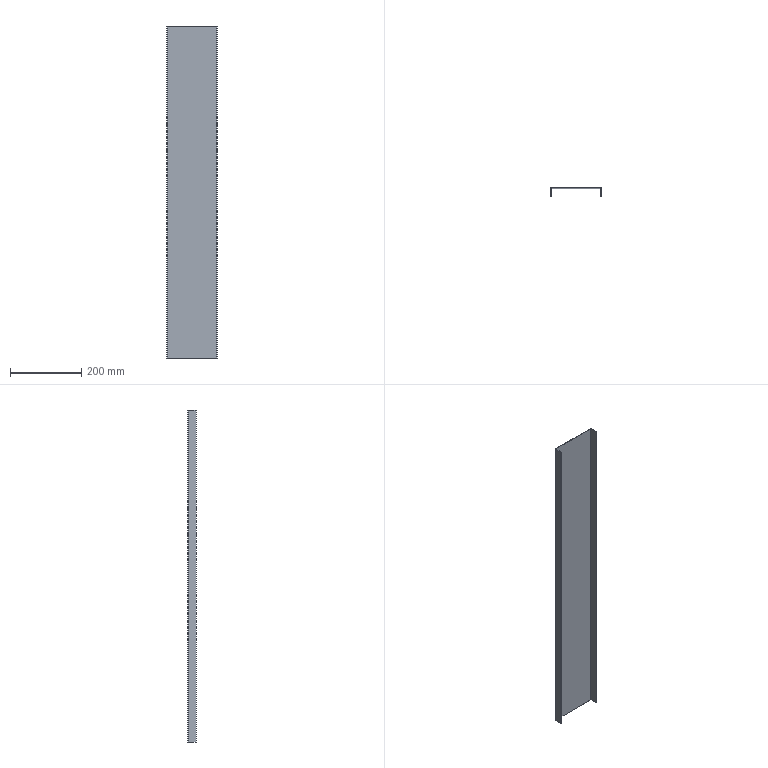Part | 1 solid | 22 faces | box 142 x 23 x 935 mm | volume 172917 mm3 | plane 18 | cylinder 4 | commonest cylinder face diameters 1.473 x2 3.473 x2
STEP:
#1=CARTESIAN_POINT('',(69.263,22.,935.));
#2=VERTEX_POINT('',#1);
#3=CARTESIAN_POINT('',(69.263,23.,935.));
#4=VERTEX_POINT('',#3);
#5=CARTESIAN_POINT('',(69.263,22.,935.));
#6=DIRECTION('',(0.,1.,0.));
#7=VECTOR('',#6,1000.);
#8=LINE('',#5,#7);
#9=EDGE_CURVE('',#2,#4,#8,.T.);
#10=ORIENTED_EDGE('',*,*,#9,.F.);
#11=CARTESIAN_POINT('',(70.,21.263,935.));
#12=VERTEX_POINT('',#11);
#13=CARTESIAN_POINT('',(69.263,21.263,935.));
#14=DIRECTION('',(0.,0.,1.));
#15=DIRECTION('',(-1.,0.,0.));
#16=AXIS2_PLACEMENT_3D('',#13,#14,#15);
#17=CIRCLE('',#16,0.7366);
#18=EDGE_CURVE('',#12,#2,#17,.T.);
#19=ORIENTED_EDGE('',*,*,#18,.F.);
#20=CARTESIAN_POINT('',(71.,21.263,935.));
#21=VERTEX_POINT('',#20);
#22=CARTESIAN_POINT('',(71.,21.263,935.));
#23=DIRECTION('',(-1.,0.,0.));
#24=VECTOR('',#23,1000.);
#25=LINE('',#22,#24);
#26=EDGE_CURVE('',#21,#12,#25,.T.);
#27=ORIENTED_EDGE('',*,*,#26,.F.);
#28=CARTESIAN_POINT('',(69.263,21.263,935.));
#29=DIRECTION('',(0.,0.,1.));
#30=DIRECTION('',(1.,0.,0.));
#31=AXIS2_PLACEMENT_3D('',#28,#29,#30);
#32=CIRCLE('',#31,1.737);
#33=EDGE_CURVE('',#21,#4,#32,.T.);
#34=ORIENTED_EDGE('',*,*,#33,.T.);
#35=EDGE_LOOP('',(#10,#19,#27,#34));
#36=FACE_OUTER_BOUND('',#35,.T.);
#37=CARTESIAN_POINT('',(69.263,22.,935.));
#38=DIRECTION('',(0.,0.,1.));
#39=DIRECTION('',(1.,0.,0.));
#40=AXIS2_PLACEMENT_3D('',#37,#38,#39);
#41=PLANE('',#40);
#42=ADVANCED_FACE('',(#36),#41,.T.);
#43=CARTESIAN_POINT('',(-69.263,22.,935.));
#44=VERTEX_POINT('',#43);
#45=CARTESIAN_POINT('',(-70.,22.,935.));
#46=DIRECTION('',(-1.,0.,0.));
#47=VECTOR('',#46,1000.);
#48=LINE('',#45,#47);
#49=EDGE_CURVE('',#2,#44,#48,.T.);
#50=ORIENTED_EDGE('',*,*,#49,.F.);
#51=ORIENTED_EDGE('',*,*,#9,.T.);
#52=CARTESIAN_POINT('',(-69.263,23.,935.));
#53=VERTEX_POINT('',#52);
#54=CARTESIAN_POINT('',(-70.,23.,935.));
#55=DIRECTION('',(-1.,0.,0.));
#56=VECTOR('',#55,1000.);
#57=LINE('',#54,#56);
#58=EDGE_CURVE('',#4,#53,#57,.T.);
#59=ORIENTED_EDGE('',*,*,#58,.T.);
#60=CARTESIAN_POINT('',(-69.263,23.,935.));
#61=DIRECTION('',(0.,-1.,0.));
#62=VECTOR('',#61,1000.);
#63=LINE('',#60,#62);
#64=EDGE_CURVE('',#53,#44,#63,.T.);
#65=ORIENTED_EDGE('',*,*,#64,.T.);
#66=EDGE_LOOP('',(#50,#51,#59,#65));
#67=FACE_OUTER_BOUND('',#66,.T.);
#68=CARTESIAN_POINT('',(71.,21.263,935.));
#69=DIRECTION('',(0.,0.,1.));
#70=DIRECTION('',(1.,0.,0.));
#71=AXIS2_PLACEMENT_3D('',#68,#69,#70);
#72=PLANE('',#71);
#73=ADVANCED_FACE('',(#67),#72,.T.);
#74=CARTESIAN_POINT('',(70.,21.263,0.));
#75=VERTEX_POINT('',#74);
#76=CARTESIAN_POINT('',(71.,21.263,0.));
#77=VERTEX_POINT('',#76);
#78=CARTESIAN_POINT('',(70.,21.263,0.));
#79=DIRECTION('',(1.,0.,0.));
#80=VECTOR('',#79,1000.);
#81=LINE('',#78,#80);
#82=EDGE_CURVE('',#75,#77,#81,.T.);
#83=ORIENTED_EDGE('',*,*,#82,.F.);
#84=CARTESIAN_POINT('',(69.263,22.,0.));
#85=VERTEX_POINT('',#84);
#86=CARTESIAN_POINT('',(69.263,21.263,0.));
#87=DIRECTION('',(0.,0.,1.));
#88=DIRECTION('',(-1.,0.,0.));
#89=AXIS2_PLACEMENT_3D('',#86,#87,#88);
#90=CIRCLE('',#89,0.7366);
#91=EDGE_CURVE('',#75,#85,#90,.T.);
#92=ORIENTED_EDGE('',*,*,#91,.T.);
#93=CARTESIAN_POINT('',(69.263,23.,0.));
#94=VERTEX_POINT('',#93);
#95=CARTESIAN_POINT('',(69.263,23.,0.));
#96=DIRECTION('',(0.,-1.,0.));
#97=VECTOR('',#96,1000.);
#98=LINE('',#95,#97);
#99=EDGE_CURVE('',#94,#85,#98,.T.);
#100=ORIENTED_EDGE('',*,*,#99,.F.);
#101=CARTESIAN_POINT('',(69.263,21.263,0.));
#102=DIRECTION('',(0.,0.,1.));
#103=DIRECTION('',(1.,0.,0.));
#104=AXIS2_PLACEMENT_3D('',#101,#102,#103);
#105=CIRCLE('',#104,1.737);
#106=EDGE_CURVE('',#77,#94,#105,.T.);
#107=ORIENTED_EDGE('',*,*,#106,.F.);
#108=EDGE_LOOP('',(#83,#92,#100,#107));
#109=FACE_OUTER_BOUND('',#108,.T.);
#110=CARTESIAN_POINT('',(70.,21.263,0.));
#111=DIRECTION('',(0.,0.,-1.));
#112=DIRECTION('',(-1.,0.,0.));
#113=AXIS2_PLACEMENT_3D('',#110,#111,#112);
#114=PLANE('',#113);
#115=ADVANCED_FACE('',(#109),#114,.T.);
#116=CARTESIAN_POINT('',(70.,0.,0.));
#117=VERTEX_POINT('',#116);
#118=CARTESIAN_POINT('',(70.,22.,0.));
#119=DIRECTION('',(0.,1.,0.));
#120=VECTOR('',#119,1000.);
#121=LINE('',#118,#120);
#122=EDGE_CURVE('',#117,#75,#121,.T.);
#123=ORIENTED_EDGE('',*,*,#122,.T.);
#124=ORIENTED_EDGE('',*,*,#82,.T.);
#125=CARTESIAN_POINT('',(71.,0.,0.));
#126=VERTEX_POINT('',#125);
#127=CARTESIAN_POINT('',(71.,22.,0.));
#128=DIRECTION('',(0.,1.,0.));
#129=VECTOR('',#128,1000.);
#130=LINE('',#127,#129);
#131=EDGE_CURVE('',#126,#77,#130,.T.);
#132=ORIENTED_EDGE('',*,*,#131,.F.);
#133=CARTESIAN_POINT('',(71.,0.,0.));
#134=DIRECTION('',(-1.,0.,0.));
#135=VECTOR('',#134,1000.);
#136=LINE('',#133,#135);
#137=EDGE_CURVE('',#126,#117,#136,.T.);
#138=ORIENTED_EDGE('',*,*,#137,.T.);
#139=EDGE_LOOP('',(#123,#124,#132,#138));
#140=FACE_OUTER_BOUND('',#139,.T.);
#141=CARTESIAN_POINT('',(69.263,23.,0.));
#142=DIRECTION('',(0.,0.,-1.));
#143=DIRECTION('',(-1.,0.,0.));
#144=AXIS2_PLACEMENT_3D('',#141,#142,#143);
#145=PLANE('',#144);
#146=ADVANCED_FACE('',(#140),#145,.T.);
#147=CARTESIAN_POINT('',(-70.,21.263,935.));
#148=VERTEX_POINT('',#147);
#149=CARTESIAN_POINT('',(-71.,21.263,935.));
#150=VERTEX_POINT('',#149);
#151=CARTESIAN_POINT('',(-70.,21.263,935.));
#152=DIRECTION('',(-1.,0.,0.));
#153=VECTOR('',#152,1000.);
#154=LINE('',#151,#153);
#155=EDGE_CURVE('',#148,#150,#154,.T.);
#156=ORIENTED_EDGE('',*,*,#155,.F.);
#157=CARTESIAN_POINT('',(-69.263,21.263,935.));
#158=DIRECTION('',(0.,0.,1.));
#159=DIRECTION('',(-1.,0.,0.));
#160=AXIS2_PLACEMENT_3D('',#157,#158,#159);
#161=CIRCLE('',#160,0.7366);
#162=EDGE_CURVE('',#44,#148,#161,.T.);
#163=ORIENTED_EDGE('',*,*,#162,.F.);
#164=ORIENTED_EDGE('',*,*,#64,.F.);
#165=CARTESIAN_POINT('',(-69.263,21.263,935.));
#166=DIRECTION('',(0.,0.,1.));
#167=DIRECTION('',(1.,0.,0.));
#168=AXIS2_PLACEMENT_3D('',#165,#166,#167);
#169=CIRCLE('',#168,1.737);
#170=EDGE_CURVE('',#53,#150,#169,.T.);
#171=ORIENTED_EDGE('',*,*,#170,.T.);
#172=EDGE_LOOP('',(#156,#163,#164,#171));
#173=FACE_OUTER_BOUND('',#172,.T.);
#174=CARTESIAN_POINT('',(-70.,21.263,935.));
#175=DIRECTION('',(0.,0.,1.));
#176=DIRECTION('',(1.,0.,0.));
#177=AXIS2_PLACEMENT_3D('',#174,#175,#176);
#178=PLANE('',#177);
#179=ADVANCED_FACE('',(#173),#178,.T.);
#180=CARTESIAN_POINT('',(-70.,0.,935.));
#181=VERTEX_POINT('',#180);
#182=CARTESIAN_POINT('',(-70.,22.,935.));
#183=DIRECTION('',(0.,-1.,0.));
#184=VECTOR('',#183,1000.);
#185=LINE('',#182,#184);
#186=EDGE_CURVE('',#148,#181,#185,.T.);
#187=ORIENTED_EDGE('',*,*,#186,.F.);
#188=ORIENTED_EDGE('',*,*,#155,.T.);
#189=CARTESIAN_POINT('',(-71.,0.,935.));
#190=VERTEX_POINT('',#189);
#191=CARTESIAN_POINT('',(-71.,22.,935.));
#192=DIRECTION('',(0.,-1.,0.));
#193=VECTOR('',#192,1000.);
#194=LINE('',#191,#193);
#195=EDGE_CURVE('',#150,#190,#194,.T.);
#196=ORIENTED_EDGE('',*,*,#195,.T.);
#197=CARTESIAN_POINT('',(-70.,0.,935.));
#198=DIRECTION('',(-1.,0.,0.));
#199=VECTOR('',#198,1000.);
#200=LINE('',#197,#199);
#201=EDGE_CURVE('',#181,#190,#200,.T.);
#202=ORIENTED_EDGE('',*,*,#201,.F.);
#203=EDGE_LOOP('',(#187,#188,#196,#202));
#204=FACE_OUTER_BOUND('',#203,.T.);
#205=CARTESIAN_POINT('',(-69.263,23.,935.));
#206=DIRECTION('',(0.,0.,1.));
#207=DIRECTION('',(1.,0.,0.));
#208=AXIS2_PLACEMENT_3D('',#205,#206,#207);
#209=PLANE('',#208);
#210=ADVANCED_FACE('',(#204),#209,.T.);
#211=CARTESIAN_POINT('',(-69.263,22.,0.));
#212=VERTEX_POINT('',#211);
#213=CARTESIAN_POINT('',(-69.263,23.,0.));
#214=VERTEX_POINT('',#213);
#215=CARTESIAN_POINT('',(-69.263,22.,0.));
#216=DIRECTION('',(0.,1.,0.));
#217=VECTOR('',#216,1000.);
#218=LINE('',#215,#217);
#219=EDGE_CURVE('',#212,#214,#218,.T.);
#220=ORIENTED_EDGE('',*,*,#219,.F.);
#221=CARTESIAN_POINT('',(-70.,21.263,0.));
#222=VERTEX_POINT('',#221);
#223=CARTESIAN_POINT('',(-69.263,21.263,0.));
#224=DIRECTION('',(0.,0.,1.));
#225=DIRECTION('',(-1.,0.,0.));
#226=AXIS2_PLACEMENT_3D('',#223,#224,#225);
#227=CIRCLE('',#226,0.7366);
#228=EDGE_CURVE('',#212,#222,#227,.T.);
#229=ORIENTED_EDGE('',*,*,#228,.T.);
#230=CARTESIAN_POINT('',(-71.,21.263,0.));
#231=VERTEX_POINT('',#230);
#232=CARTESIAN_POINT('',(-71.,21.263,0.));
#233=DIRECTION('',(1.,0.,0.));
#234=VECTOR('',#233,1000.);
#235=LINE('',#232,#234);
#236=EDGE_CURVE('',#231,#222,#235,.T.);
#237=ORIENTED_EDGE('',*,*,#236,.F.);
#238=CARTESIAN_POINT('',(-69.263,21.263,0.));
#239=DIRECTION('',(0.,0.,1.));
#240=DIRECTION('',(1.,0.,0.));
#241=AXIS2_PLACEMENT_3D('',#238,#239,#240);
#242=CIRCLE('',#241,1.737);
#243=EDGE_CURVE('',#214,#231,#242,.T.);
#244=ORIENTED_EDGE('',*,*,#243,.F.);
#245=EDGE_LOOP('',(#220,#229,#237,#244));
#246=FACE_OUTER_BOUND('',#245,.T.);
#247=CARTESIAN_POINT('',(-69.263,22.,0.));
#248=DIRECTION('',(0.,0.,-1.));
#249=DIRECTION('',(-1.,0.,0.));
#250=AXIS2_PLACEMENT_3D('',#247,#248,#249);
#251=PLANE('',#250);
#252=ADVANCED_FACE('',(#246),#251,.T.);
#253=CARTESIAN_POINT('',(-70.,22.,0.));
#254=DIRECTION('',(-1.,0.,0.));
#255=VECTOR('',#254,1000.);
#256=LINE('',#253,#255);
#257=EDGE_CURVE('',#85,#212,#256,.T.);
#258=ORIENTED_EDGE('',*,*,#257,.T.);
#259=ORIENTED_EDGE('',*,*,#219,.T.);
#260=CARTESIAN_POINT('',(-70.,23.,0.));
#261=DIRECTION('',(-1.,0.,0.));
#262=VECTOR('',#261,1000.);
#263=LINE('',#260,#262);
#264=EDGE_CURVE('',#94,#214,#263,.T.);
#265=ORIENTED_EDGE('',*,*,#264,.F.);
#266=ORIENTED_EDGE('',*,*,#99,.T.);
#267=EDGE_LOOP('',(#258,#259,#265,#266));
#268=FACE_OUTER_BOUND('',#267,.T.);
#269=CARTESIAN_POINT('',(-71.,21.263,0.));
#270=DIRECTION('',(0.,0.,-1.));
#271=DIRECTION('',(-1.,0.,0.));
#272=AXIS2_PLACEMENT_3D('',#269,#270,#271);
#273=PLANE('',#272);
#274=ADVANCED_FACE('',(#268),#273,.T.);
#275=CARTESIAN_POINT('',(-71.,0.,0.));
#276=VERTEX_POINT('',#275);
#277=CARTESIAN_POINT('',(-71.,22.,0.));
#278=DIRECTION('',(0.,-1.,0.));
#279=VECTOR('',#278,1000.);
#280=LINE('',#277,#279);
#281=EDGE_CURVE('',#231,#276,#280,.T.);
#282=ORIENTED_EDGE('',*,*,#281,.T.);
#283=CARTESIAN_POINT('',(-71.,0.,935.));
#284=DIRECTION('',(0.,0.,-1.));
#285=VECTOR('',#284,1000.);
#286=LINE('',#283,#285);
#287=EDGE_CURVE('',#190,#276,#286,.T.);
#288=ORIENTED_EDGE('',*,*,#287,.F.);
#289=ORIENTED_EDGE('',*,*,#195,.F.);
#290=CARTESIAN_POINT('',(-71.,21.263,935.));
#291=DIRECTION('',(0.,0.,-1.));
#292=VECTOR('',#291,1000.);
#293=LINE('',#290,#292);
#294=EDGE_CURVE('',#150,#231,#293,.T.);
#295=ORIENTED_EDGE('',*,*,#294,.T.);
#296=EDGE_LOOP('',(#282,#288,#289,#295));
#297=FACE_OUTER_BOUND('',#296,.T.);
#298=CARTESIAN_POINT('',(-71.,22.,935.));
#299=DIRECTION('',(1.,0.,0.));
#300=DIRECTION('',(0.,0.,-1.));
#301=AXIS2_PLACEMENT_3D('',#298,#299,#300);
#302=PLANE('',#301);
#303=ADVANCED_FACE('',(#297),#302,.F.);
#304=CARTESIAN_POINT('',(-70.,0.,0.));
#305=VERTEX_POINT('',#304);
#306=CARTESIAN_POINT('',(-70.,0.,0.));
#307=DIRECTION('',(-1.,0.,0.));
#308=VECTOR('',#307,1000.);
#309=LINE('',#306,#308);
#310=EDGE_CURVE('',#305,#276,#309,.T.);
#311=ORIENTED_EDGE('',*,*,#310,.F.);
#312=CARTESIAN_POINT('',(-70.,0.,935.));
#313=DIRECTION('',(0.,0.,-1.));
#314=VECTOR('',#313,1000.);
#315=LINE('',#312,#314);
#316=EDGE_CURVE('',#181,#305,#315,.T.);
#317=ORIENTED_EDGE('',*,*,#316,.F.);
#318=ORIENTED_EDGE('',*,*,#201,.T.);
#319=ORIENTED_EDGE('',*,*,#287,.T.);
#320=EDGE_LOOP('',(#311,#317,#318,#319));
#321=FACE_OUTER_BOUND('',#320,.T.);
#322=CARTESIAN_POINT('',(-70.,0.,935.));
#323=DIRECTION('',(0.,-1.,0.));
#324=DIRECTION('',(0.,0.,-1.));
#325=AXIS2_PLACEMENT_3D('',#322,#323,#324);
#326=PLANE('',#325);
#327=ADVANCED_FACE('',(#321),#326,.T.);
#328=CARTESIAN_POINT('',(-70.,22.,0.));
#329=DIRECTION('',(0.,-1.,0.));
#330=VECTOR('',#329,1000.);
#331=LINE('',#328,#330);
#332=EDGE_CURVE('',#222,#305,#331,.T.);
#333=ORIENTED_EDGE('',*,*,#332,.F.);
#334=CARTESIAN_POINT('',(-70.,21.263,935.));
#335=DIRECTION('',(0.,0.,-1.));
#336=VECTOR('',#335,1000.);
#337=LINE('',#334,#336);
#338=EDGE_CURVE('',#148,#222,#337,.T.);
#339=ORIENTED_EDGE('',*,*,#338,.F.);
#340=ORIENTED_EDGE('',*,*,#186,.T.);
#341=ORIENTED_EDGE('',*,*,#316,.T.);
#342=EDGE_LOOP('',(#333,#339,#340,#341));
#343=FACE_OUTER_BOUND('',#342,.T.);
#344=CARTESIAN_POINT('',(-70.,22.,935.));
#345=DIRECTION('',(1.,0.,0.));
#346=DIRECTION('',(0.,0.,-1.));
#347=AXIS2_PLACEMENT_3D('',#344,#345,#346);
#348=PLANE('',#347);
#349=ADVANCED_FACE('',(#343),#348,.T.);
#350=ORIENTED_EDGE('',*,*,#228,.F.);
#351=CARTESIAN_POINT('',(-69.263,22.,935.));
#352=DIRECTION('',(0.,0.,-1.));
#353=VECTOR('',#352,1000.);
#354=LINE('',#351,#353);
#355=EDGE_CURVE('',#44,#212,#354,.T.);
#356=ORIENTED_EDGE('',*,*,#355,.F.);
#357=ORIENTED_EDGE('',*,*,#162,.T.);
#358=ORIENTED_EDGE('',*,*,#338,.T.);
#359=EDGE_LOOP('',(#350,#356,#357,#358));
#360=FACE_OUTER_BOUND('',#359,.T.);
#361=CARTESIAN_POINT('',(-69.263,21.263,935.));
#362=DIRECTION('',(0.,0.,-1.));
#363=DIRECTION('',(-1.,0.,0.));
#364=AXIS2_PLACEMENT_3D('',#361,#362,#363);
#365=CYLINDRICAL_SURFACE('',#364,0.7366);
#366=ADVANCED_FACE('',(#360),#365,.F.);
#367=ORIENTED_EDGE('',*,*,#257,.F.);
#368=CARTESIAN_POINT('',(69.263,22.,935.));
#369=DIRECTION('',(0.,0.,-1.));
#370=VECTOR('',#369,1000.);
#371=LINE('',#368,#370);
#372=EDGE_CURVE('',#2,#85,#371,.T.);
#373=ORIENTED_EDGE('',*,*,#372,.F.);
#374=ORIENTED_EDGE('',*,*,#49,.T.);
#375=ORIENTED_EDGE('',*,*,#355,.T.);
#376=EDGE_LOOP('',(#367,#373,#374,#375));
#377=FACE_OUTER_BOUND('',#376,.T.);
#378=CARTESIAN_POINT('',(-70.,22.,935.));
#379=DIRECTION('',(0.,-1.,0.));
#380=DIRECTION('',(0.,0.,-1.));
#381=AXIS2_PLACEMENT_3D('',#378,#379,#380);
#382=PLANE('',#381);
#383=ADVANCED_FACE('',(#377),#382,.T.);
#384=ORIENTED_EDGE('',*,*,#91,.F.);
#385=CARTESIAN_POINT('',(70.,21.263,935.));
#386=DIRECTION('',(0.,0.,-1.));
#387=VECTOR('',#386,1000.);
#388=LINE('',#385,#387);
#389=EDGE_CURVE('',#12,#75,#388,.T.);
#390=ORIENTED_EDGE('',*,*,#389,.F.);
#391=ORIENTED_EDGE('',*,*,#18,.T.);
#392=ORIENTED_EDGE('',*,*,#372,.T.);
#393=EDGE_LOOP('',(#384,#390,#391,#392));
#394=FACE_OUTER_BOUND('',#393,.T.);
#395=CARTESIAN_POINT('',(69.263,21.263,935.));
#396=DIRECTION('',(0.,0.,-1.));
#397=DIRECTION('',(-1.,0.,0.));
#398=AXIS2_PLACEMENT_3D('',#395,#396,#397);
#399=CYLINDRICAL_SURFACE('',#398,0.7366);
#400=ADVANCED_FACE('',(#394),#399,.F.);
#401=ORIENTED_EDGE('',*,*,#122,.F.);
#402=CARTESIAN_POINT('',(70.,0.,935.));
#403=VERTEX_POINT('',#402);
#404=CARTESIAN_POINT('',(70.,0.,935.));
#405=DIRECTION('',(0.,0.,-1.));
#406=VECTOR('',#405,1000.);
#407=LINE('',#404,#406);
#408=EDGE_CURVE('',#403,#117,#407,.T.);
#409=ORIENTED_EDGE('',*,*,#408,.F.);
#410=CARTESIAN_POINT('',(70.,22.,935.));
#411=DIRECTION('',(0.,1.,0.));
#412=VECTOR('',#411,1000.);
#413=LINE('',#410,#412);
#414=EDGE_CURVE('',#403,#12,#413,.T.);
#415=ORIENTED_EDGE('',*,*,#414,.T.);
#416=ORIENTED_EDGE('',*,*,#389,.T.);
#417=EDGE_LOOP('',(#401,#409,#415,#416));
#418=FACE_OUTER_BOUND('',#417,.T.);
#419=CARTESIAN_POINT('',(70.,22.,935.));
#420=DIRECTION('',(-1.,0.,0.));
#421=DIRECTION('',(0.,0.,1.));
#422=AXIS2_PLACEMENT_3D('',#419,#420,#421);
#423=PLANE('',#422);
#424=ADVANCED_FACE('',(#418),#423,.T.);
#425=ORIENTED_EDGE('',*,*,#137,.F.);
#426=CARTESIAN_POINT('',(71.,0.,935.));
#427=VERTEX_POINT('',#426);
#428=CARTESIAN_POINT('',(71.,0.,935.));
#429=DIRECTION('',(0.,0.,-1.));
#430=VECTOR('',#429,1000.);
#431=LINE('',#428,#430);
#432=EDGE_CURVE('',#427,#126,#431,.T.);
#433=ORIENTED_EDGE('',*,*,#432,.F.);
#434=CARTESIAN_POINT('',(71.,0.,935.));
#435=DIRECTION('',(-1.,0.,0.));
#436=VECTOR('',#435,1000.);
#437=LINE('',#434,#436);
#438=EDGE_CURVE('',#427,#403,#437,.T.);
#439=ORIENTED_EDGE('',*,*,#438,.T.);
#440=ORIENTED_EDGE('',*,*,#408,.T.);
#441=EDGE_LOOP('',(#425,#433,#439,#440));
#442=FACE_OUTER_BOUND('',#441,.T.);
#443=CARTESIAN_POINT('',(71.,0.,935.));
#444=DIRECTION('',(0.,-1.,0.));
#445=DIRECTION('',(0.,0.,-1.));
#446=AXIS2_PLACEMENT_3D('',#443,#444,#445);
#447=PLANE('',#446);
#448=ADVANCED_FACE('',(#442),#447,.T.);
#449=ORIENTED_EDGE('',*,*,#131,.T.);
#450=CARTESIAN_POINT('',(71.,21.263,935.));
#451=DIRECTION('',(0.,0.,-1.));
#452=VECTOR('',#451,1000.);
#453=LINE('',#450,#452);
#454=EDGE_CURVE('',#21,#77,#453,.T.);
#455=ORIENTED_EDGE('',*,*,#454,.F.);
#456=CARTESIAN_POINT('',(71.,22.,935.));
#457=DIRECTION('',(0.,1.,0.));
#458=VECTOR('',#457,1000.);
#459=LINE('',#456,#458);
#460=EDGE_CURVE('',#427,#21,#459,.T.);
#461=ORIENTED_EDGE('',*,*,#460,.F.);
#462=ORIENTED_EDGE('',*,*,#432,.T.);
#463=EDGE_LOOP('',(#449,#455,#461,#462));
#464=FACE_OUTER_BOUND('',#463,.T.);
#465=CARTESIAN_POINT('',(71.,22.,935.));
#466=DIRECTION('',(-1.,0.,0.));
#467=DIRECTION('',(0.,0.,1.));
#468=AXIS2_PLACEMENT_3D('',#465,#466,#467);
#469=PLANE('',#468);
#470=ADVANCED_FACE('',(#464),#469,.F.);
#471=ORIENTED_EDGE('',*,*,#106,.T.);
#472=CARTESIAN_POINT('',(69.263,23.,935.));
#473=DIRECTION('',(0.,0.,-1.));
#474=VECTOR('',#473,1000.);
#475=LINE('',#472,#474);
#476=EDGE_CURVE('',#4,#94,#475,.T.);
#477=ORIENTED_EDGE('',*,*,#476,.F.);
#478=ORIENTED_EDGE('',*,*,#33,.F.);
#479=ORIENTED_EDGE('',*,*,#454,.T.);
#480=EDGE_LOOP('',(#471,#477,#478,#479));
#481=FACE_OUTER_BOUND('',#480,.T.);
#482=CARTESIAN_POINT('',(69.263,21.263,935.));
#483=DIRECTION('',(0.,0.,-1.));
#484=DIRECTION('',(-1.,0.,0.));
#485=AXIS2_PLACEMENT_3D('',#482,#483,#484);
#486=CYLINDRICAL_SURFACE('',#485,1.737);
#487=ADVANCED_FACE('',(#481),#486,.T.);
#488=ORIENTED_EDGE('',*,*,#264,.T.);
#489=CARTESIAN_POINT('',(-69.263,23.,935.));
#490=DIRECTION('',(0.,0.,-1.));
#491=VECTOR('',#490,1000.);
#492=LINE('',#489,#491);
#493=EDGE_CURVE('',#53,#214,#492,.T.);
#494=ORIENTED_EDGE('',*,*,#493,.F.);
#495=ORIENTED_EDGE('',*,*,#58,.F.);
#496=ORIENTED_EDGE('',*,*,#476,.T.);
#497=EDGE_LOOP('',(#488,#494,#495,#496));
#498=FACE_OUTER_BOUND('',#497,.T.);
#499=CARTESIAN_POINT('',(-70.,23.,935.));
#500=DIRECTION('',(0.,-1.,0.));
#501=DIRECTION('',(0.,0.,-1.));
#502=AXIS2_PLACEMENT_3D('',#499,#500,#501);
#503=PLANE('',#502);
#504=ADVANCED_FACE('',(#498),#503,.F.);
#505=ORIENTED_EDGE('',*,*,#243,.T.);
#506=ORIENTED_EDGE('',*,*,#294,.F.);
#507=ORIENTED_EDGE('',*,*,#170,.F.);
#508=ORIENTED_EDGE('',*,*,#493,.T.);
#509=EDGE_LOOP('',(#505,#506,#507,#508));
#510=FACE_OUTER_BOUND('',#509,.T.);
#511=CARTESIAN_POINT('',(-69.263,21.263,935.));
#512=DIRECTION('',(0.,0.,-1.));
#513=DIRECTION('',(-1.,0.,0.));
#514=AXIS2_PLACEMENT_3D('',#511,#512,#513);
#515=CYLINDRICAL_SURFACE('',#514,1.737);
#516=ADVANCED_FACE('',(#510),#515,.T.);
#517=ORIENTED_EDGE('',*,*,#460,.T.);
#518=ORIENTED_EDGE('',*,*,#26,.T.);
#519=ORIENTED_EDGE('',*,*,#414,.F.);
#520=ORIENTED_EDGE('',*,*,#438,.F.);
#521=EDGE_LOOP('',(#517,#518,#519,#520));
#522=FACE_OUTER_BOUND('',#521,.T.);
#523=CARTESIAN_POINT('',(-69.263,21.263,935.));
#524=DIRECTION('',(0.,0.,-1.));
#525=DIRECTION('',(-1.,0.,0.));
#526=AXIS2_PLACEMENT_3D('',#523,#524,#525);
#527=PLANE('',#526);
#528=ADVANCED_FACE('',(#522),#527,.F.);
#529=ORIENTED_EDGE('',*,*,#281,.F.);
#530=ORIENTED_EDGE('',*,*,#236,.T.);
#531=ORIENTED_EDGE('',*,*,#332,.T.);
#532=ORIENTED_EDGE('',*,*,#310,.T.);
#533=EDGE_LOOP('',(#529,#530,#531,#532));
#534=FACE_OUTER_BOUND('',#533,.T.);
#535=CARTESIAN_POINT('',(-69.263,21.263,0.));
#536=DIRECTION('',(0.,0.,-1.));
#537=DIRECTION('',(-1.,0.,0.));
#538=AXIS2_PLACEMENT_3D('',#535,#536,#537);
#539=PLANE('',#538);
#540=ADVANCED_FACE('',(#534),#539,.T.);
#541=CLOSED_SHELL('',(#42,#73,#115,#146,#179,#210,#252,#274,#303,#327,#349,#366,#383,#400,#424,#448,#470,#487,#504,#516,#528,#540));
#542=MANIFOLD_SOLID_BREP('',#541);
#543=CARTESIAN_POINT('',(0.,0.,0.));
#544=DIRECTION('',(0.,0.,1.));
#545=DIRECTION('',(1.,0.,0.));
#546=AXIS2_PLACEMENT_3D('',#543,#544,#545);
#547=(LENGTH_UNIT()NAMED_UNIT(*)SI_UNIT(.MILLI.,.METRE.));
#548=UNCERTAINTY_MEASURE_WITH_UNIT(LENGTH_MEASURE(0.00001),#547,'','');
#549=(NAMED_UNIT(*)PLANE_ANGLE_UNIT()SI_UNIT($,.RADIAN.));
#550=(NAMED_UNIT(*)SI_UNIT($,.STERADIAN.)SOLID_ANGLE_UNIT());
#551=(GEOMETRIC_REPRESENTATION_CONTEXT(3)GLOBAL_UNCERTAINTY_ASSIGNED_CONTEXT((#548))GLOBAL_UNIT_ASSIGNED_CONTEXT((#547,#549,#550))REPRESENTATION_CONTEXT('',''));
#552=ADVANCED_BREP_SHAPE_REPRESENTATION('',(#542,#546),#551);